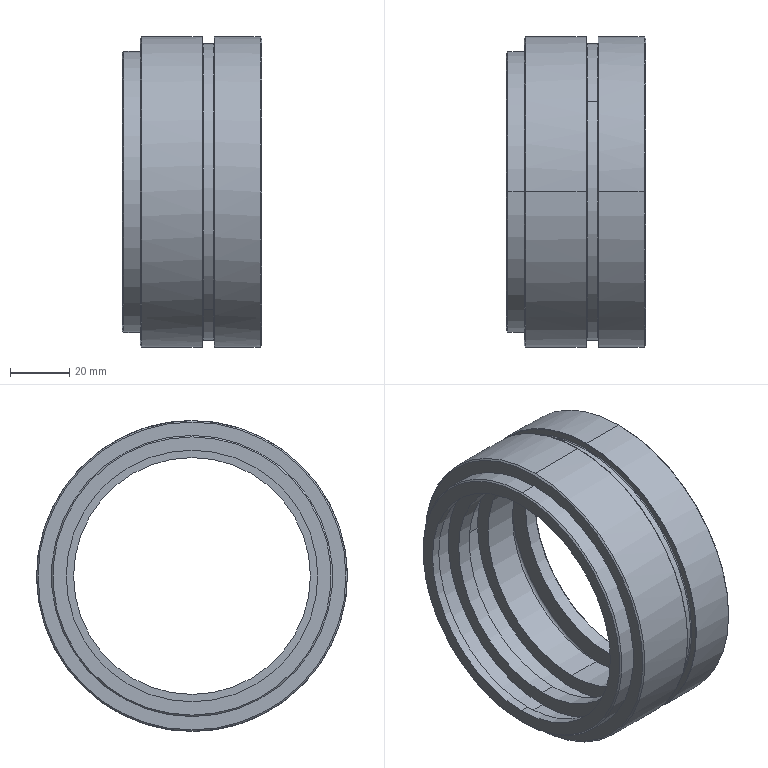Part | SolidWorks | features Cavity 1, Chamfer 1, Extrusion 1, ICE 1 | 1 solid | 53 faces | box 47 x 105 x 105 mm | volume 121428 mm3 | cylinder 22 | torus 12 | plane 11 | cone 8 | commonest cylinder face diameters 80 x6 90 x4 105 x4 85 x2 95 x2 95.5 x2
STEP:
#1=CARTESIAN_POINT('',(35.7,0.,-40.));
#2=VERTEX_POINT('',#1);
#3=CARTESIAN_POINT('',(35.7,0.,40.));
#4=VERTEX_POINT('',#3);
#5=CARTESIAN_POINT('',(35.7,0.000000867,0.000001335));
#6=DIRECTION('',(-1.,0.,0.));
#7=DIRECTION('',(0.,-0.1106,0.9939));
#8=AXIS2_PLACEMENT_3D('',#5,#6,#7);
#9=CIRCLE('',#8,40.);
#10=EDGE_CURVE('',#2,#4,#9,.T.);
#11=ORIENTED_EDGE('',*,*,#10,.F.);
#12=CARTESIAN_POINT('',(24.,0.,-40.));
#13=VERTEX_POINT('',#12);
#14=CARTESIAN_POINT('',(47.,0.,-40.));
#15=DIRECTION('',(-1.,0.,0.));
#16=VECTOR('',#15,1000.);
#17=LINE('',#14,#16);
#18=EDGE_CURVE('',#2,#13,#17,.T.);
#19=ORIENTED_EDGE('',*,*,#18,.T.);
#20=CARTESIAN_POINT('',(24.,0.,40.));
#21=VERTEX_POINT('',#20);
#22=CARTESIAN_POINT('',(24.,0.000000867,0.000001335));
#23=DIRECTION('',(-1.,0.,0.));
#24=DIRECTION('',(0.,-0.9995,0.03037));
#25=AXIS2_PLACEMENT_3D('',#22,#23,#24);
#26=CIRCLE('',#25,40.);
#27=EDGE_CURVE('',#13,#21,#26,.T.);
#28=ORIENTED_EDGE('',*,*,#27,.T.);
#29=CARTESIAN_POINT('',(47.,0.,40.));
#30=DIRECTION('',(-1.,0.,0.));
#31=VECTOR('',#30,1000.);
#32=LINE('',#29,#31);
#33=EDGE_CURVE('',#4,#21,#32,.T.);
#34=ORIENTED_EDGE('',*,*,#33,.F.);
#35=EDGE_LOOP('',(#11,#19,#28,#34));
#36=FACE_OUTER_BOUND('',#35,.T.);
#37=CARTESIAN_POINT('',(47.,0.,0.));
#38=DIRECTION('',(-1.,0.,0.));
#39=DIRECTION('',(0.,0.,1.));
#40=AXIS2_PLACEMENT_3D('',#37,#38,#39);
#41=CYLINDRICAL_SURFACE('',#40,40.);
#42=ADVANCED_FACE('',(#36),#41,.F.);
#43=CARTESIAN_POINT('',(24.,44.979,-1.366));
#44=VERTEX_POINT('',#43);
#45=CARTESIAN_POINT('',(24.,-44.979,1.366));
#46=VERTEX_POINT('',#45);
#47=CARTESIAN_POINT('',(24.,0.000000867,0.000001335));
#48=DIRECTION('',(-1.,0.,0.));
#49=DIRECTION('',(0.,-0.9995,0.03037));
#50=AXIS2_PLACEMENT_3D('',#47,#48,#49);
#51=CIRCLE('',#50,45.);
#52=EDGE_CURVE('',#44,#46,#51,.T.);
#53=ORIENTED_EDGE('',*,*,#52,.F.);
#54=CARTESIAN_POINT('',(15.,44.979,-1.366));
#55=VERTEX_POINT('',#54);
#56=CARTESIAN_POINT('',(15.,44.979,-1.366));
#57=DIRECTION('',(-1.,0.,0.));
#58=VECTOR('',#57,1000.);
#59=LINE('',#56,#58);
#60=EDGE_CURVE('',#44,#55,#59,.T.);
#61=ORIENTED_EDGE('',*,*,#60,.T.);
#62=CARTESIAN_POINT('',(15.,-44.979,1.366));
#63=VERTEX_POINT('',#62);
#64=CARTESIAN_POINT('',(15.,0.000000867,0.000001335));
#65=DIRECTION('',(-1.,0.,0.));
#66=DIRECTION('',(0.,-0.9995,0.03037));
#67=AXIS2_PLACEMENT_3D('',#64,#65,#66);
#68=CIRCLE('',#67,45.);
#69=EDGE_CURVE('',#55,#63,#68,.T.);
#70=ORIENTED_EDGE('',*,*,#69,.T.);
#71=CARTESIAN_POINT('',(15.,-44.979,1.366));
#72=DIRECTION('',(-1.,0.,0.));
#73=VECTOR('',#72,1000.);
#74=LINE('',#71,#73);
#75=EDGE_CURVE('',#46,#63,#74,.T.);
#76=ORIENTED_EDGE('',*,*,#75,.F.);
#77=EDGE_LOOP('',(#53,#61,#70,#76));
#78=FACE_OUTER_BOUND('',#77,.T.);
#79=CARTESIAN_POINT('',(15.,0.000000867,0.000001335));
#80=DIRECTION('',(-1.,0.,0.));
#81=DIRECTION('',(0.,-0.9995,0.03037));
#82=AXIS2_PLACEMENT_3D('',#79,#80,#81);
#83=CYLINDRICAL_SURFACE('',#82,45.);
#84=ADVANCED_FACE('',(#78),#83,.F.);
#85=CARTESIAN_POINT('',(36.7,5.281,-47.457));
#86=VERTEX_POINT('',#85);
#87=CARTESIAN_POINT('',(36.7,-5.281,47.457));
#88=VERTEX_POINT('',#87);
#89=CARTESIAN_POINT('',(36.7,0.000000867,0.000001335));
#90=DIRECTION('',(-1.,0.,0.));
#91=DIRECTION('',(0.,-0.1106,0.9939));
#92=AXIS2_PLACEMENT_3D('',#89,#90,#91);
#93=CIRCLE('',#92,47.75);
#94=EDGE_CURVE('',#86,#88,#93,.T.);
#95=ORIENTED_EDGE('',*,*,#94,.F.);
#96=CARTESIAN_POINT('',(35.7,5.171,-46.463));
#97=VERTEX_POINT('',#96);
#98=CARTESIAN_POINT('',(36.7,5.171,-46.463));
#99=DIRECTION('',(0.,0.9939,0.1106));
#100=DIRECTION('',(0.,-0.1106,0.9939));
#101=AXIS2_PLACEMENT_3D('',#98,#99,#100);
#102=CIRCLE('',#101,1.);
#103=EDGE_CURVE('',#86,#97,#102,.T.);
#104=ORIENTED_EDGE('',*,*,#103,.T.);
#105=CARTESIAN_POINT('',(35.7,-5.171,46.463));
#106=VERTEX_POINT('',#105);
#107=CARTESIAN_POINT('',(35.7,0.000000867,0.000001335));
#108=DIRECTION('',(-1.,0.,0.));
#109=DIRECTION('',(0.,-0.1106,0.9939));
#110=AXIS2_PLACEMENT_3D('',#107,#108,#109);
#111=CIRCLE('',#110,46.75);
#112=EDGE_CURVE('',#97,#106,#111,.T.);
#113=ORIENTED_EDGE('',*,*,#112,.T.);
#114=CARTESIAN_POINT('',(36.7,-5.171,46.463));
#115=DIRECTION('',(0.,-0.9939,-0.1106));
#116=DIRECTION('',(0.,0.1106,-0.9939));
#117=AXIS2_PLACEMENT_3D('',#114,#115,#116);
#118=CIRCLE('',#117,1.);
#119=EDGE_CURVE('',#88,#106,#118,.T.);
#120=ORIENTED_EDGE('',*,*,#119,.F.);
#121=EDGE_LOOP('',(#95,#104,#113,#120));
#122=FACE_OUTER_BOUND('',#121,.T.);
#123=CARTESIAN_POINT('',(36.7,0.000000867,0.000001335));
#124=DIRECTION('',(-1.,0.,0.));
#125=DIRECTION('',(0.,-0.1106,0.9939));
#126=AXIS2_PLACEMENT_3D('',#123,#124,#125);
#127=TOROIDAL_SURFACE('',#126,46.75,1.);
#128=ADVANCED_FACE('',(#122),#127,.F.);
#129=CARTESIAN_POINT('',(41.,5.281,-47.457));
#130=VERTEX_POINT('',#129);
#131=CARTESIAN_POINT('',(41.,-5.281,47.457));
#132=VERTEX_POINT('',#131);
#133=CARTESIAN_POINT('',(41.,0.000000867,0.000001335));
#134=DIRECTION('',(-1.,0.,0.));
#135=DIRECTION('',(0.,-0.1106,0.9939));
#136=AXIS2_PLACEMENT_3D('',#133,#134,#135);
#137=CIRCLE('',#136,47.75);
#138=EDGE_CURVE('',#130,#132,#137,.T.);
#139=ORIENTED_EDGE('',*,*,#138,.F.);
#140=CARTESIAN_POINT('',(35.7,5.281,-47.457));
#141=DIRECTION('',(-1.,0.,0.));
#142=VECTOR('',#141,1000.);
#143=LINE('',#140,#142);
#144=EDGE_CURVE('',#130,#86,#143,.T.);
#145=ORIENTED_EDGE('',*,*,#144,.T.);
#146=ORIENTED_EDGE('',*,*,#94,.T.);
#147=CARTESIAN_POINT('',(35.7,-5.281,47.457));
#148=DIRECTION('',(-1.,0.,0.));
#149=VECTOR('',#148,1000.);
#150=LINE('',#147,#149);
#151=EDGE_CURVE('',#132,#88,#150,.T.);
#152=ORIENTED_EDGE('',*,*,#151,.F.);
#153=EDGE_LOOP('',(#139,#145,#146,#152));
#154=FACE_OUTER_BOUND('',#153,.T.);
#155=CARTESIAN_POINT('',(35.7,0.000000867,0.000001335));
#156=DIRECTION('',(-1.,0.,0.));
#157=DIRECTION('',(0.,-0.1106,0.9939));
#158=AXIS2_PLACEMENT_3D('',#155,#156,#157);
#159=CYLINDRICAL_SURFACE('',#158,47.75);
#160=ADVANCED_FACE('',(#154),#159,.F.);
#161=CARTESIAN_POINT('',(42.,5.171,-46.463));
#162=VERTEX_POINT('',#161);
#163=CARTESIAN_POINT('',(42.,-5.171,46.463));
#164=VERTEX_POINT('',#163);
#165=CARTESIAN_POINT('',(42.,0.000000867,0.000001335));
#166=DIRECTION('',(-1.,0.,0.));
#167=DIRECTION('',(0.,-0.1106,0.9939));
#168=AXIS2_PLACEMENT_3D('',#165,#166,#167);
#169=CIRCLE('',#168,46.75);
#170=EDGE_CURVE('',#162,#164,#169,.T.);
#171=ORIENTED_EDGE('',*,*,#170,.F.);
#172=CARTESIAN_POINT('',(41.,5.171,-46.463));
#173=DIRECTION('',(0.,0.9939,0.1106));
#174=DIRECTION('',(0.,-0.1106,0.9939));
#175=AXIS2_PLACEMENT_3D('',#172,#173,#174);
#176=CIRCLE('',#175,1.);
#177=EDGE_CURVE('',#162,#130,#176,.T.);
#178=ORIENTED_EDGE('',*,*,#177,.T.);
#179=ORIENTED_EDGE('',*,*,#138,.T.);
#180=CARTESIAN_POINT('',(41.,-5.171,46.463));
#181=DIRECTION('',(0.,-0.9939,-0.1106));
#182=DIRECTION('',(0.,0.1106,-0.9939));
#183=AXIS2_PLACEMENT_3D('',#180,#181,#182);
#184=CIRCLE('',#183,1.);
#185=EDGE_CURVE('',#164,#132,#184,.T.);
#186=ORIENTED_EDGE('',*,*,#185,.F.);
#187=EDGE_LOOP('',(#171,#178,#179,#186));
#188=FACE_OUTER_BOUND('',#187,.T.);
#189=CARTESIAN_POINT('',(41.,0.000000867,0.000001335));
#190=DIRECTION('',(-1.,0.,0.));
#191=DIRECTION('',(0.,-0.1106,0.9939));
#192=AXIS2_PLACEMENT_3D('',#189,#190,#191);
#193=TOROIDAL_SURFACE('',#192,46.75,1.);
#194=ADVANCED_FACE('',(#188),#193,.F.);
#195=CARTESIAN_POINT('',(46.5,0.,40.));
#196=VERTEX_POINT('',#195);
#197=CARTESIAN_POINT('',(46.5,0.,-40.));
#198=VERTEX_POINT('',#197);
#199=CARTESIAN_POINT('',(46.5,0.,0.));
#200=DIRECTION('',(1.,0.,0.));
#201=DIRECTION('',(0.,0.,-1.));
#202=AXIS2_PLACEMENT_3D('',#199,#200,#201);
#203=CIRCLE('',#202,40.);
#204=EDGE_CURVE('',#196,#198,#203,.T.);
#205=ORIENTED_EDGE('',*,*,#204,.T.);
#206=CARTESIAN_POINT('',(42.,0.,-40.));
#207=VERTEX_POINT('',#206);
#208=CARTESIAN_POINT('',(47.,0.,-40.));
#209=DIRECTION('',(-1.,0.,0.));
#210=VECTOR('',#209,1000.);
#211=LINE('',#208,#210);
#212=EDGE_CURVE('',#198,#207,#211,.T.);
#213=ORIENTED_EDGE('',*,*,#212,.T.);
#214=CARTESIAN_POINT('',(42.,0.,40.));
#215=VERTEX_POINT('',#214);
#216=CARTESIAN_POINT('',(42.,0.000000867,0.000001335));
#217=DIRECTION('',(-1.,0.,0.));
#218=DIRECTION('',(0.,-0.1106,0.9939));
#219=AXIS2_PLACEMENT_3D('',#216,#217,#218);
#220=CIRCLE('',#219,40.);
#221=EDGE_CURVE('',#207,#215,#220,.T.);
#222=ORIENTED_EDGE('',*,*,#221,.T.);
#223=CARTESIAN_POINT('',(47.,0.,40.));
#224=DIRECTION('',(-1.,0.,0.));
#225=VECTOR('',#224,1000.);
#226=LINE('',#223,#225);
#227=EDGE_CURVE('',#196,#215,#226,.T.);
#228=ORIENTED_EDGE('',*,*,#227,.F.);
#229=EDGE_LOOP('',(#205,#213,#222,#228));
#230=FACE_OUTER_BOUND('',#229,.T.);
#231=CARTESIAN_POINT('',(47.,0.,0.));
#232=DIRECTION('',(-1.,0.,0.));
#233=DIRECTION('',(0.,0.,1.));
#234=AXIS2_PLACEMENT_3D('',#231,#232,#233);
#235=CYLINDRICAL_SURFACE('',#234,40.);
#236=ADVANCED_FACE('',(#230),#235,.F.);
#237=ORIENTED_EDGE('',*,*,#204,.F.);
#238=CARTESIAN_POINT('',(47.,0.,40.5));
#239=VERTEX_POINT('',#238);
#240=CARTESIAN_POINT('',(46.5,0.,40.));
#241=DIRECTION('',(0.7071,0.,0.7071));
#242=VECTOR('',#241,1000.);
#243=LINE('',#240,#242);
#244=EDGE_CURVE('',#196,#239,#243,.T.);
#245=ORIENTED_EDGE('',*,*,#244,.T.);
#246=CARTESIAN_POINT('',(47.,0.,-40.5));
#247=VERTEX_POINT('',#246);
#248=CARTESIAN_POINT('',(47.,0.,0.));
#249=DIRECTION('',(-1.,0.,0.));
#250=DIRECTION('',(0.,0.,-1.));
#251=AXIS2_PLACEMENT_3D('',#248,#249,#250);
#252=CIRCLE('',#251,40.5);
#253=EDGE_CURVE('',#247,#239,#252,.T.);
#254=ORIENTED_EDGE('',*,*,#253,.F.);
#255=CARTESIAN_POINT('',(46.5,0.,-40.));
#256=DIRECTION('',(0.7071,0.,-0.7071));
#257=VECTOR('',#256,1000.);
#258=LINE('',#255,#257);
#259=EDGE_CURVE('',#198,#247,#258,.T.);
#260=ORIENTED_EDGE('',*,*,#259,.F.);
#261=EDGE_LOOP('',(#237,#245,#254,#260));
#262=FACE_OUTER_BOUND('',#261,.T.);
#263=CARTESIAN_POINT('',(46.5,0.,0.));
#264=DIRECTION('',(1.,0.,0.));
#265=DIRECTION('',(0.,0.,-1.));
#266=AXIS2_PLACEMENT_3D('',#263,#264,#265);
#267=CONICAL_SURFACE('',#266,40.,0.7854);
#268=ADVANCED_FACE('',(#262),#267,.F.);
#269=CARTESIAN_POINT('',(46.5,0.,52.5));
#270=VERTEX_POINT('',#269);
#271=CARTESIAN_POINT('',(46.5,0.,-52.5));
#272=VERTEX_POINT('',#271);
#273=CARTESIAN_POINT('',(46.5,0.,0.));
#274=DIRECTION('',(-1.,0.,0.));
#275=DIRECTION('',(0.,0.,-1.));
#276=AXIS2_PLACEMENT_3D('',#273,#274,#275);
#277=CIRCLE('',#276,52.5);
#278=EDGE_CURVE('',#270,#272,#277,.T.);
#279=ORIENTED_EDGE('',*,*,#278,.T.);
#280=CARTESIAN_POINT('',(31.1,0.,-52.5));
#281=VERTEX_POINT('',#280);
#282=CARTESIAN_POINT('',(47.,0.,-52.5));
#283=DIRECTION('',(-1.,0.,0.));
#284=VECTOR('',#283,1000.);
#285=LINE('',#282,#284);
#286=EDGE_CURVE('',#272,#281,#285,.T.);
#287=ORIENTED_EDGE('',*,*,#286,.T.);
#288=CARTESIAN_POINT('',(31.1,31.96,41.651));
#289=VERTEX_POINT('',#288);
#290=CARTESIAN_POINT('',(31.1,0.,0.));
#291=DIRECTION('',(1.,0.,0.));
#292=DIRECTION('',(0.,-0.6088,-0.7934));
#293=AXIS2_PLACEMENT_3D('',#290,#291,#292);
#294=CIRCLE('',#293,52.5);
#295=EDGE_CURVE('',#281,#289,#294,.T.);
#296=ORIENTED_EDGE('',*,*,#295,.T.);
#297=CARTESIAN_POINT('',(31.1,0.,52.5));
#298=VERTEX_POINT('',#297);
#299=CARTESIAN_POINT('',(31.1,0.,0.));
#300=DIRECTION('',(1.,0.,0.));
#301=DIRECTION('',(0.,-0.6088,-0.7934));
#302=AXIS2_PLACEMENT_3D('',#299,#300,#301);
#303=CIRCLE('',#302,52.5);
#304=EDGE_CURVE('',#289,#298,#303,.T.);
#305=ORIENTED_EDGE('',*,*,#304,.T.);
#306=CARTESIAN_POINT('',(47.,0.,52.5));
#307=DIRECTION('',(-1.,0.,0.));
#308=VECTOR('',#307,1000.);
#309=LINE('',#306,#308);
#310=EDGE_CURVE('',#270,#298,#309,.T.);
#311=ORIENTED_EDGE('',*,*,#310,.F.);
#312=EDGE_LOOP('',(#279,#287,#296,#305,#311));
#313=FACE_OUTER_BOUND('',#312,.T.);
#314=CARTESIAN_POINT('',(47.,0.,0.));
#315=DIRECTION('',(-1.,0.,0.));
#316=DIRECTION('',(0.,0.,1.));
#317=AXIS2_PLACEMENT_3D('',#314,#315,#316);
#318=CYLINDRICAL_SURFACE('',#317,52.5);
#319=ADVANCED_FACE('',(#313),#318,.T.);
#320=CARTESIAN_POINT('',(47.,0.,-52.));
#321=VERTEX_POINT('',#320);
#322=CARTESIAN_POINT('',(47.,0.,52.));
#323=VERTEX_POINT('',#322);
#324=CARTESIAN_POINT('',(47.,0.,0.));
#325=DIRECTION('',(1.,0.,0.));
#326=DIRECTION('',(0.,0.,-1.));
#327=AXIS2_PLACEMENT_3D('',#324,#325,#326);
#328=CIRCLE('',#327,52.);
#329=EDGE_CURVE('',#321,#323,#328,.T.);
#330=ORIENTED_EDGE('',*,*,#329,.F.);
#331=CARTESIAN_POINT('',(47.,0.,-52.));
#332=DIRECTION('',(-0.7071,0.,-0.7071));
#333=VECTOR('',#332,1000.);
#334=LINE('',#331,#333);
#335=EDGE_CURVE('',#321,#272,#334,.T.);
#336=ORIENTED_EDGE('',*,*,#335,.T.);
#337=ORIENTED_EDGE('',*,*,#278,.F.);
#338=CARTESIAN_POINT('',(47.,0.,52.));
#339=DIRECTION('',(-0.7071,0.,0.7071));
#340=VECTOR('',#339,1000.);
#341=LINE('',#338,#340);
#342=EDGE_CURVE('',#323,#270,#341,.T.);
#343=ORIENTED_EDGE('',*,*,#342,.F.);
#344=EDGE_LOOP('',(#330,#336,#337,#343));
#345=FACE_OUTER_BOUND('',#344,.T.);
#346=CARTESIAN_POINT('',(47.,0.,0.));
#347=DIRECTION('',(-1.,0.,0.));
#348=DIRECTION('',(0.,0.,1.));
#349=AXIS2_PLACEMENT_3D('',#346,#347,#348);
#350=CONICAL_SURFACE('',#349,52.,0.7854);
#351=ADVANCED_FACE('',(#345),#350,.T.);
#352=CARTESIAN_POINT('',(15.,0.,-40.));
#353=VERTEX_POINT('',#352);
#354=CARTESIAN_POINT('',(15.,0.,40.));
#355=VERTEX_POINT('',#354);
#356=CARTESIAN_POINT('',(15.,0.000000867,0.000001335));
#357=DIRECTION('',(-1.,0.,0.));
#358=DIRECTION('',(0.,-0.9995,0.03037));
#359=AXIS2_PLACEMENT_3D('',#356,#357,#358);
#360=CIRCLE('',#359,40.);
#361=EDGE_CURVE('',#353,#355,#360,.T.);
#362=ORIENTED_EDGE('',*,*,#361,.F.);
#363=CARTESIAN_POINT('',(10.,0.,-40.));
#364=VERTEX_POINT('',#363);
#365=CARTESIAN_POINT('',(47.,0.,-40.));
#366=DIRECTION('',(-1.,0.,0.));
#367=VECTOR('',#366,1000.);
#368=LINE('',#365,#367);
#369=EDGE_CURVE('',#353,#364,#368,.T.);
#370=ORIENTED_EDGE('',*,*,#369,.T.);
#371=CARTESIAN_POINT('',(10.,0.,40.));
#372=VERTEX_POINT('',#371);
#373=CARTESIAN_POINT('',(10.,0.,0.));
#374=DIRECTION('',(-1.,0.,0.));
#375=DIRECTION('',(0.,0.,1.));
#376=AXIS2_PLACEMENT_3D('',#373,#374,#375);
#377=CIRCLE('',#376,40.);
#378=EDGE_CURVE('',#364,#372,#377,.T.);
#379=ORIENTED_EDGE('',*,*,#378,.T.);
#380=CARTESIAN_POINT('',(47.,0.,40.));
#381=DIRECTION('',(-1.,0.,0.));
#382=VECTOR('',#381,1000.);
#383=LINE('',#380,#382);
#384=EDGE_CURVE('',#355,#372,#383,.T.);
#385=ORIENTED_EDGE('',*,*,#384,.F.);
#386=EDGE_LOOP('',(#362,#370,#379,#385));
#387=FACE_OUTER_BOUND('',#386,.T.);
#388=CARTESIAN_POINT('',(47.,0.,0.));
#389=DIRECTION('',(-1.,0.,0.));
#390=DIRECTION('',(0.,0.,1.));
#391=AXIS2_PLACEMENT_3D('',#388,#389,#390);
#392=CYLINDRICAL_SURFACE('',#391,40.);
#393=ADVANCED_FACE('',(#387),#392,.F.);
#394=CARTESIAN_POINT('',(31.,-31.899,-41.572));
#395=VERTEX_POINT('',#394);
#396=CARTESIAN_POINT('',(31.,31.899,41.572));
#397=VERTEX_POINT('',#396);
#398=CARTESIAN_POINT('',(31.,0.,0.));
#399=DIRECTION('',(1.,0.,0.));
#400=DIRECTION('',(0.,-0.6088,-0.7934));
#401=AXIS2_PLACEMENT_3D('',#398,#399,#400);
#402=CIRCLE('',#401,52.4);
#403=EDGE_CURVE('',#395,#397,#402,.T.);
#404=ORIENTED_EDGE('',*,*,#403,.T.);
#405=CARTESIAN_POINT('',(31.1,31.899,41.572));
#406=DIRECTION('',(0.,0.7934,-0.6088));
#407=DIRECTION('',(0.,0.6088,0.7934));
#408=AXIS2_PLACEMENT_3D('',#405,#406,#407);
#409=CIRCLE('',#408,0.1);
#410=EDGE_CURVE('',#397,#289,#409,.T.);
#411=ORIENTED_EDGE('',*,*,#410,.T.);
#412=ORIENTED_EDGE('',*,*,#295,.F.);
#413=CARTESIAN_POINT('',(31.1,-31.96,-41.651));
#414=VERTEX_POINT('',#413);
#415=CARTESIAN_POINT('',(31.1,0.,0.));
#416=DIRECTION('',(1.,0.,0.));
#417=DIRECTION('',(0.,-0.6088,-0.7934));
#418=AXIS2_PLACEMENT_3D('',#415,#416,#417);
#419=CIRCLE('',#418,52.5);
#420=EDGE_CURVE('',#414,#281,#419,.T.);
#421=ORIENTED_EDGE('',*,*,#420,.F.);
#422=CARTESIAN_POINT('',(31.1,-31.899,-41.572));
#423=DIRECTION('',(0.,-0.7934,0.6088));
#424=DIRECTION('',(0.,-0.6088,-0.7934));
#425=AXIS2_PLACEMENT_3D('',#422,#423,#424);
#426=CIRCLE('',#425,0.1);
#427=EDGE_CURVE('',#395,#414,#426,.T.);
#428=ORIENTED_EDGE('',*,*,#427,.F.);
#429=EDGE_LOOP('',(#404,#411,#412,#421,#428));
#430=FACE_OUTER_BOUND('',#429,.T.);
#431=CARTESIAN_POINT('',(31.1,0.,0.));
#432=DIRECTION('',(1.,0.,0.));
#433=DIRECTION('',(0.,-0.6088,-0.7934));
#434=AXIS2_PLACEMENT_3D('',#431,#432,#433);
#435=TOROIDAL_SURFACE('',#434,52.4,0.1);
#436=ADVANCED_FACE('',(#430),#435,.T.);
#437=CARTESIAN_POINT('',(26.9,0.,-52.5));
#438=VERTEX_POINT('',#437);
#439=CARTESIAN_POINT('',(26.9,31.96,41.651));
#440=VERTEX_POINT('',#439);
#441=CARTESIAN_POINT('',(26.9,0.,0.));
#442=DIRECTION('',(1.,0.,0.));
#443=DIRECTION('',(0.,-0.6088,-0.7934));
#444=AXIS2_PLACEMENT_3D('',#441,#442,#443);
#445=CIRCLE('',#444,52.5);
#446=EDGE_CURVE('',#438,#440,#445,.T.);
#447=ORIENTED_EDGE('',*,*,#446,.T.);
#448=CARTESIAN_POINT('',(27.,31.899,41.572));
#449=VERTEX_POINT('',#448);
#450=CARTESIAN_POINT('',(26.9,31.899,41.572));
#451=DIRECTION('',(0.,0.7934,-0.6088));
#452=DIRECTION('',(0.,0.6088,0.7934));
#453=AXIS2_PLACEMENT_3D('',#450,#451,#452);
#454=CIRCLE('',#453,0.1);
#455=EDGE_CURVE('',#440,#449,#454,.T.);
#456=ORIENTED_EDGE('',*,*,#455,.T.);
#457=CARTESIAN_POINT('',(27.,-31.899,-41.572));
#458=VERTEX_POINT('',#457);
#459=CARTESIAN_POINT('',(27.,0.,0.));
#460=DIRECTION('',(1.,0.,0.));
#461=DIRECTION('',(0.,-0.6088,-0.7934));
#462=AXIS2_PLACEMENT_3D('',#459,#460,#461);
#463=CIRCLE('',#462,52.4);
#464=EDGE_CURVE('',#458,#449,#463,.T.);
#465=ORIENTED_EDGE('',*,*,#464,.F.);
#466=CARTESIAN_POINT('',(26.9,-31.96,-41.651));
#467=VERTEX_POINT('',#466);
#468=CARTESIAN_POINT('',(26.9,-31.899,-41.572));
#469=DIRECTION('',(0.,-0.7934,0.6088));
#470=DIRECTION('',(0.,-0.6088,-0.7934));
#471=AXIS2_PLACEMENT_3D('',#468,#469,#470);
#472=CIRCLE('',#471,0.1);
#473=EDGE_CURVE('',#467,#458,#472,.T.);
#474=ORIENTED_EDGE('',*,*,#473,.F.);
#475=CARTESIAN_POINT('',(26.9,0.,0.));
#476=DIRECTION('',(1.,0.,0.));
#477=DIRECTION('',(0.,-0.6088,-0.7934));
#478=AXIS2_PLACEMENT_3D('',#475,#476,#477);
#479=CIRCLE('',#478,52.5);
#480=EDGE_CURVE('',#467,#438,#479,.T.);
#481=ORIENTED_EDGE('',*,*,#480,.T.);
#482=EDGE_LOOP('',(#447,#456,#465,#474,#481));
#483=FACE_OUTER_BOUND('',#482,.T.);
#484=CARTESIAN_POINT('',(26.9,0.,0.));
#485=DIRECTION('',(1.,0.,0.));
#486=DIRECTION('',(0.,-0.6088,-0.7934));
#487=AXIS2_PLACEMENT_3D('',#484,#485,#486);
#488=TOROIDAL_SURFACE('',#487,52.4,0.1);
#489=ADVANCED_FACE('',(#483),#488,.T.);
#490=CARTESIAN_POINT('',(27.3,30.499,39.747));
#491=VERTEX_POINT('',#490);
#492=CARTESIAN_POINT('',(27.3,-30.499,-39.747));
#493=VERTEX_POINT('',#492);
#494=CARTESIAN_POINT('',(27.3,0.,0.));
#495=DIRECTION('',(1.,0.,0.));
#496=DIRECTION('',(0.,-0.6088,-0.7934));
#497=AXIS2_PLACEMENT_3D('',#494,#495,#496);
#498=CIRCLE('',#497,50.1);
#499=EDGE_CURVE('',#491,#493,#498,.T.);
#500=ORIENTED_EDGE('',*,*,#499,.F.);
#501=CARTESIAN_POINT('',(27.,30.681,39.985));
#502=VERTEX_POINT('',#501);
#503=CARTESIAN_POINT('',(27.3,30.681,39.985));
#504=DIRECTION('',(0.,0.7934,-0.6088));
#505=DIRECTION('',(0.,0.6088,0.7934));
#506=AXIS2_PLACEMENT_3D('',#503,#504,#505);
#507=CIRCLE('',#506,0.3);
#508=EDGE_CURVE('',#491,#502,#507,.T.);
#509=ORIENTED_EDGE('',*,*,#508,.T.);
#510=CARTESIAN_POINT('',(27.,-30.681,-39.985));
#511=VERTEX_POINT('',#510);
#512=CARTESIAN_POINT('',(27.,0.,0.));
#513=DIRECTION('',(1.,0.,0.));
#514=DIRECTION('',(0.,-0.6088,-0.7934));
#515=AXIS2_PLACEMENT_3D('',#512,#513,#514);
#516=CIRCLE('',#515,50.4);
#517=EDGE_CURVE('',#502,#511,#516,.T.);
#518=ORIENTED_EDGE('',*,*,#517,.T.);
#519=CARTESIAN_POINT('',(27.3,-30.681,-39.985));
#520=DIRECTION('',(0.,-0.7934,0.6088));
#521=DIRECTION('',(0.,-0.6088,-0.7934));
#522=AXIS2_PLACEMENT_3D('',#519,#520,#521);
#523=CIRCLE('',#522,0.3);
#524=EDGE_CURVE('',#493,#511,#523,.T.);
#525=ORIENTED_EDGE('',*,*,#524,.F.);
#526=EDGE_LOOP('',(#500,#509,#518,#525));
#527=FACE_OUTER_BOUND('',#526,.T.);
#528=CARTESIAN_POINT('',(27.3,0.,0.));
#529=DIRECTION('',(1.,0.,0.));
#530=DIRECTION('',(0.,-0.6088,-0.7934));
#531=AXIS2_PLACEMENT_3D('',#528,#529,#530);
#532=TOROIDAL_SURFACE('',#531,50.4,0.3);
#533=ADVANCED_FACE('',(#527),#532,.F.);
#534=CARTESIAN_POINT('',(27.3,0.,0.));
#535=DIRECTION('',(1.,0.,0.));
#536=DIRECTION('',(0.,-0.6088,-0.7934));
#537=AXIS2_PLACEMENT_3D('',#534,#535,#536);
#538=CIRCLE('',#537,50.1);
#539=EDGE_CURVE('',#493,#491,#538,.T.);
#540=ORIENTED_EDGE('',*,*,#539,.T.);
#541=CARTESIAN_POINT('',(30.7,30.499,39.747));
#542=VERTEX_POINT('',#541);
#543=CARTESIAN_POINT('',(196.04,30.499,39.747));
#544=DIRECTION('',(1.,0.,0.));
#545=VECTOR('',#544,1000.);
#546=LINE('',#543,#545);
#547=EDGE_CURVE('',#491,#542,#546,.T.);
#548=ORIENTED_EDGE('',*,*,#547,.T.);
#549=CARTESIAN_POINT('',(30.7,-30.499,-39.747));
#550=VERTEX_POINT('',#549);
#551=CARTESIAN_POINT('',(30.7,0.,0.));
#552=DIRECTION('',(1.,0.,0.));
#553=DIRECTION('',(0.,-0.6088,-0.7934));
#554=AXIS2_PLACEMENT_3D('',#551,#552,#553);
#555=CIRCLE('',#554,50.1);
#556=EDGE_CURVE('',#550,#542,#555,.T.);
#557=ORIENTED_EDGE('',*,*,#556,.F.);
#558=CARTESIAN_POINT('',(196.04,-30.499,-39.747));
#559=DIRECTION('',(1.,0.,0.));
#560=VECTOR('',#559,1000.);
#561=LINE('',#558,#560);
#562=EDGE_CURVE('',#493,#550,#561,.T.);
#563=ORIENTED_EDGE('',*,*,#562,.F.);
#564=EDGE_LOOP('',(#540,#548,#557,#563));
#565=FACE_OUTER_BOUND('',#564,.T.);
#566=CARTESIAN_POINT('',(196.04,0.,0.));
#567=DIRECTION('',(1.,0.,0.));
#568=DIRECTION('',(0.,-0.6088,-0.7934));
#569=AXIS2_PLACEMENT_3D('',#566,#567,#568);
#570=CYLINDRICAL_SURFACE('',#569,50.1);
#571=ADVANCED_FACE('',(#565),#570,.T.);
#572=CARTESIAN_POINT('',(31.,30.681,39.985));
#573=VERTEX_POINT('',#572);
#574=CARTESIAN_POINT('',(31.,-30.681,-39.985));
#575=VERTEX_POINT('',#574);
#576=CARTESIAN_POINT('',(31.,0.,0.));
#577=DIRECTION('',(1.,0.,0.));
#578=DIRECTION('',(0.,-0.6088,-0.7934));
#579=AXIS2_PLACEMENT_3D('',#576,#577,#578);
#580=CIRCLE('',#579,50.4);
#581=EDGE_CURVE('',#573,#575,#580,.T.);
#582=ORIENTED_EDGE('',*,*,#581,.F.);
#583=CARTESIAN_POINT('',(30.7,30.681,39.985));
#584=DIRECTION('',(0.,0.7934,-0.6088));
#585=DIRECTION('',(0.,0.6088,0.7934));
#586=AXIS2_PLACEMENT_3D('',#583,#584,#585);
#587=CIRCLE('',#586,0.3);
#588=EDGE_CURVE('',#573,#542,#587,.T.);
#589=ORIENTED_EDGE('',*,*,#588,.T.);
#590=CARTESIAN_POINT('',(30.7,0.,0.));
#591=DIRECTION('',(1.,0.,0.));
#592=DIRECTION('',(0.,-0.6088,-0.7934));
#593=AXIS2_PLACEMENT_3D('',#590,#591,#592);
#594=CIRCLE('',#593,50.1);
#595=EDGE_CURVE('',#542,#550,#594,.T.);
#596=ORIENTED_EDGE('',*,*,#595,.T.);
#597=CARTESIAN_POINT('',(30.7,-30.681,-39.985));
#598=DIRECTION('',(0.,-0.7934,0.6088));
#599=DIRECTION('',(0.,-0.6088,-0.7934));
#600=AXIS2_PLACEMENT_3D('',#597,#598,#599);
#601=CIRCLE('',#600,0.3);
#602=EDGE_CURVE('',#575,#550,#601,.T.);
#603=ORIENTED_EDGE('',*,*,#602,.F.);
#604=EDGE_LOOP('',(#582,#589,#596,#603));
#605=FACE_OUTER_BOUND('',#604,.T.);
#606=CARTESIAN_POINT('',(30.7,0.,0.));
#607=DIRECTION('',(1.,0.,0.));
#608=DIRECTION('',(0.,-0.6088,-0.7934));
#609=AXIS2_PLACEMENT_3D('',#606,#607,#608);
#610=TOROIDAL_SURFACE('',#609,50.4,0.3);
#611=ADVANCED_FACE('',(#605),#610,.F.);
#612=CARTESIAN_POINT('',(10.,0.,-45.));
#613=VERTEX_POINT('',#612);
#614=CARTESIAN_POINT('',(10.,0.,45.));
#615=VERTEX_POINT('',#614);
#616=CARTESIAN_POINT('',(10.,0.,0.));
#617=DIRECTION('',(-1.,0.,0.));
#618=DIRECTION('',(0.,0.,1.));
#619=AXIS2_PLACEMENT_3D('',#616,#617,#618);
#620=CIRCLE('',#619,45.);
#621=EDGE_CURVE('',#613,#615,#620,.T.);
#622=ORIENTED_EDGE('',*,*,#621,.F.);
#623=CARTESIAN_POINT('',(3.,0.,-45.));
#624=VERTEX_POINT('',#623);
#625=CARTESIAN_POINT('',(-2.,0.,-45.));
#626=DIRECTION('',(-1.,0.,0.));
#627=VECTOR('',#626,1000.);
#628=LINE('',#625,#627);
#629=EDGE_CURVE('',#613,#624,#628,.T.);
#630=ORIENTED_EDGE('',*,*,#629,.T.);
#631=CARTESIAN_POINT('',(3.,0.,45.));
#632=VERTEX_POINT('',#631);
#633=CARTESIAN_POINT('',(3.,0.,0.));
#634=DIRECTION('',(-1.,0.,0.));
#635=DIRECTION('',(0.,0.,1.));
#636=AXIS2_PLACEMENT_3D('',#633,#634,#635);
#637=CIRCLE('',#636,45.);
#638=EDGE_CURVE('',#624,#632,#637,.T.);
#639=ORIENTED_EDGE('',*,*,#638,.T.);
#640=CARTESIAN_POINT('',(-2.,0.,45.));
#641=DIRECTION('',(-1.,0.,0.));
#642=VECTOR('',#641,1000.);
#643=LINE('',#640,#642);
#644=EDGE_CURVE('',#615,#632,#643,.T.);
#645=ORIENTED_EDGE('',*,*,#644,.F.);
#646=EDGE_LOOP('',(#622,#630,#639,#645));
#647=FACE_OUTER_BOUND('',#646,.T.);
#648=CARTESIAN_POINT('',(-2.,0.,0.));
#649=DIRECTION('',(-1.,0.,0.));
#650=DIRECTION('',(0.,0.,1.));
#651=AXIS2_PLACEMENT_3D('',#648,#649,#650);
#652=CYLINDRICAL_SURFACE('',#651,45.);
#653=ADVANCED_FACE('',(#647),#652,.F.);
#654=CARTESIAN_POINT('',(3.,0.,-42.5));
#655=VERTEX_POINT('',#654);
#656=CARTESIAN_POINT('',(3.,0.,42.5));
#657=VERTEX_POINT('',#656);
#658=CARTESIAN_POINT('',(3.,0.,0.));
#659=DIRECTION('',(-1.,0.,0.));
#660=DIRECTION('',(0.,0.,1.));
#661=AXIS2_PLACEMENT_3D('',#658,#659,#660);
#662=CIRCLE('',#661,42.5);
#663=EDGE_CURVE('',#655,#657,#662,.T.);
#664=ORIENTED_EDGE('',*,*,#663,.F.);
#665=CARTESIAN_POINT('',(0.,0.,-42.5));
#666=VERTEX_POINT('',#665);
#667=CARTESIAN_POINT('',(-2.,0.,-42.5));
#668=DIRECTION('',(-1.,0.,0.));
#669=VECTOR('',#668,1000.);
#670=LINE('',#667,#669);
#671=EDGE_CURVE('',#655,#666,#670,.T.);
#672=ORIENTED_EDGE('',*,*,#671,.T.);
#673=CARTESIAN_POINT('',(0.,0.,42.5));
#674=VERTEX_POINT('',#673);
#675=CARTESIAN_POINT('',(0.,0.,0.));
#676=DIRECTION('',(-1.,0.,0.));
#677=DIRECTION('',(0.,0.,-1.));
#678=AXIS2_PLACEMENT_3D('',#675,#676,#677);
#679=CIRCLE('',#678,42.5);
#680=EDGE_CURVE('',#666,#674,#679,.T.);
#681=ORIENTED_EDGE('',*,*,#680,.T.);
#682=CARTESIAN_POINT('',(-2.,0.,42.5));
#683=DIRECTION('',(-1.,0.,0.));
#684=VECTOR('',#683,1000.);
#685=LINE('',#682,#684);
#686=EDGE_CURVE('',#657,#674,#685,.T.);
#687=ORIENTED_EDGE('',*,*,#686,.F.);
#688=EDGE_LOOP('',(#664,#672,#681,#687));
#689=FACE_OUTER_BOUND('',#688,.T.);
#690=CARTESIAN_POINT('',(-2.,0.,0.));
#691=DIRECTION('',(-1.,0.,0.));
#692=DIRECTION('',(0.,0.,1.));
#693=AXIS2_PLACEMENT_3D('',#690,#691,#692);
#694=CYLINDRICAL_SURFACE('',#693,42.5);
#695=ADVANCED_FACE('',(#689),#694,.F.);
#696=CARTESIAN_POINT('',(0.,0.,47.));
#697=VERTEX_POINT('',#696);
#698=CARTESIAN_POINT('',(0.,0.,-47.));
#699=VERTEX_POINT('',#698);
#700=CARTESIAN_POINT('',(0.,0.,0.));
#701=DIRECTION('',(-1.,0.,0.));
#702=DIRECTION('',(0.,0.,-1.));
#703=AXIS2_PLACEMENT_3D('',#700,#701,#702);
#704=CIRCLE('',#703,47.);
#705=EDGE_CURVE('',#697,#699,#704,.T.);
#706=ORIENTED_EDGE('',*,*,#705,.F.);
#707=CARTESIAN_POINT('',(0.5,0.,47.5));
#708=VERTEX_POINT('',#707);
#709=CARTESIAN_POINT('',(0.,0.,47.));
#710=DIRECTION('',(0.7071,0.,0.7071));
#711=VECTOR('',#710,1000.);
#712=LINE('',#709,#711);
#713=EDGE_CURVE('',#697,#708,#712,.T.);
#714=ORIENTED_EDGE('',*,*,#713,.T.);
#715=CARTESIAN_POINT('',(0.5,0.,-47.5));
#716=VERTEX_POINT('',#715);
#717=CARTESIAN_POINT('',(0.5,0.,0.));
#718=DIRECTION('',(1.,0.,0.));
#719=DIRECTION('',(0.,0.,-1.));
#720=AXIS2_PLACEMENT_3D('',#717,#718,#719);
#721=CIRCLE('',#720,47.5);
#722=EDGE_CURVE('',#716,#708,#721,.T.);
#723=ORIENTED_EDGE('',*,*,#722,.F.);
#724=CARTESIAN_POINT('',(0.,0.,-47.));
#725=DIRECTION('',(0.7071,0.,-0.7071));
#726=VECTOR('',#725,1000.);
#727=LINE('',#724,#726);
#728=EDGE_CURVE('',#699,#716,#727,.T.);
#729=ORIENTED_EDGE('',*,*,#728,.F.);
#730=EDGE_LOOP('',(#706,#714,#723,#729));
#731=FACE_OUTER_BOUND('',#730,.T.);
#732=CARTESIAN_POINT('',(0.,0.,0.));
#733=DIRECTION('',(1.,0.,0.));
#734=DIRECTION('',(0.,0.,-1.));
#735=AXIS2_PLACEMENT_3D('',#732,#733,#734);
#736=CONICAL_SURFACE('',#735,47.,0.7854);
#737=ADVANCED_FACE('',(#731),#736,.T.);
#738=CARTESIAN_POINT('',(6.,0.,52.));
#739=VERTEX_POINT('',#738);
#740=CARTESIAN_POINT('',(6.,0.,-52.));
#741=VERTEX_POINT('',#740);
#742=CARTESIAN_POINT('',(6.,0.,0.));
#743=DIRECTION('',(-1.,0.,0.));
#744=DIRECTION('',(0.,0.,1.));
#745=AXIS2_PLACEMENT_3D('',#742,#743,#744);
#746=CIRCLE('',#745,52.);
#747=EDGE_CURVE('',#739,#741,#746,.T.);
#748=ORIENTED_EDGE('',*,*,#747,.F.);
#749=CARTESIAN_POINT('',(6.5,0.,52.5));
#750=VERTEX_POINT('',#749);
#751=CARTESIAN_POINT('',(6.,0.,52.));
#752=DIRECTION('',(0.7071,0.,0.7071));
#753=VECTOR('',#752,1000.);
#754=LINE('',#751,#753);
#755=EDGE_CURVE('',#739,#750,#754,.T.);
#756=ORIENTED_EDGE('',*,*,#755,.T.);
#757=CARTESIAN_POINT('',(6.5,0.,-52.5));
#758=VERTEX_POINT('',#757);
#759=CARTESIAN_POINT('',(6.5,0.,0.));
#760=DIRECTION('',(1.,0.,0.));
#761=DIRECTION('',(0.,0.,1.));
#762=AXIS2_PLACEMENT_3D('',#759,#760,#761);
#763=CIRCLE('',#762,52.5);
#764=EDGE_CURVE('',#758,#750,#763,.T.);
#765=ORIENTED_EDGE('',*,*,#764,.F.);
#766=CARTESIAN_POINT('',(6.,0.,-52.));
#767=DIRECTION('',(0.7071,0.,-0.7071));
#768=VECTOR('',#767,1000.);
#769=LINE('',#766,#768);
#770=EDGE_CURVE('',#741,#758,#769,.T.);
#771=ORIENTED_EDGE('',*,*,#770,.F.);
#772=EDGE_LOOP('',(#748,#756,#765,#771));
#773=FACE_OUTER_BOUND('',#772,.T.);
#774=CARTESIAN_POINT('',(6.,0.,0.));
#775=DIRECTION('',(1.,0.,0.));
#776=DIRECTION('',(0.,0.,-1.));
#777=AXIS2_PLACEMENT_3D('',#774,#775,#776);
#778=CONICAL_SURFACE('',#777,52.,0.7854);
#779=ADVANCED_FACE('',(#773),#778,.T.);
#780=CARTESIAN_POINT('',(6.,0.,47.5));
#781=VERTEX_POINT('',#780);
#782=CARTESIAN_POINT('',(6.,0.,-47.5));
#783=VERTEX_POINT('',#782);
#784=CARTESIAN_POINT('',(6.,0.,0.));
#785=DIRECTION('',(-1.,0.,0.));
#786=DIRECTION('',(0.,0.,1.));
#787=AXIS2_PLACEMENT_3D('',#784,#785,#786);
#788=CIRCLE('',#787,47.5);
#789=EDGE_CURVE('',#781,#783,#788,.T.);
#790=ORIENTED_EDGE('',*,*,#789,.T.);
#791=CARTESIAN_POINT('',(6.,0.,-47.5));
#792=DIRECTION('',(-1.,0.,0.));
#793=VECTOR('',#792,1000.);
#794=LINE('',#791,#793);
#795=EDGE_CURVE('',#783,#716,#794,.T.);
#796=ORIENTED_EDGE('',*,*,#795,.T.);
#797=ORIENTED_EDGE('',*,*,#722,.T.);
#798=CARTESIAN_POINT('',(6.,0.,47.5));
#799=DIRECTION('',(-1.,0.,0.));
#800=VECTOR('',#799,1000.);
#801=LINE('',#798,#800);
#802=EDGE_CURVE('',#781,#708,#801,.T.);
#803=ORIENTED_EDGE('',*,*,#802,.F.);
#804=EDGE_LOOP('',(#790,#796,#797,#803));
#805=FACE_OUTER_BOUND('',#804,.T.);
#806=CARTESIAN_POINT('',(6.,0.,0.));
#807=DIRECTION('',(-1.,0.,0.));
#808=DIRECTION('',(0.,0.,1.));
#809=AXIS2_PLACEMENT_3D('',#806,#807,#808);
#810=CYLINDRICAL_SURFACE('',#809,47.5);
#811=ADVANCED_FACE('',(#805),#810,.T.);
#812=ORIENTED_EDGE('',*,*,#446,.F.);
#813=CARTESIAN_POINT('',(47.,0.,-52.5));
#814=DIRECTION('',(-1.,0.,0.));
#815=VECTOR('',#814,1000.);
#816=LINE('',#813,#815);
#817=EDGE_CURVE('',#438,#758,#816,.T.);
#818=ORIENTED_EDGE('',*,*,#817,.T.);
#819=ORIENTED_EDGE('',*,*,#764,.T.);
#820=CARTESIAN_POINT('',(26.9,0.,52.5));
#821=VERTEX_POINT('',#820);
#822=CARTESIAN_POINT('',(47.,0.,52.5));
#823=DIRECTION('',(-1.,0.,0.));
#824=VECTOR('',#823,1000.);
#825=LINE('',#822,#824);
#826=EDGE_CURVE('',#821,#750,#825,.T.);
#827=ORIENTED_EDGE('',*,*,#826,.F.);
#828=CARTESIAN_POINT('',(26.9,0.,0.));
#829=DIRECTION('',(1.,0.,0.));
#830=DIRECTION('',(0.,-0.6088,-0.7934));
#831=AXIS2_PLACEMENT_3D('',#828,#829,#830);
#832=CIRCLE('',#831,52.5);
#833=EDGE_CURVE('',#440,#821,#832,.T.);
#834=ORIENTED_EDGE('',*,*,#833,.F.);
#835=EDGE_LOOP('',(#812,#818,#819,#827,#834));
#836=FACE_OUTER_BOUND('',#835,.T.);
#837=CARTESIAN_POINT('',(47.,0.,0.));
#838=DIRECTION('',(-1.,0.,0.));
#839=DIRECTION('',(0.,0.,1.));
#840=AXIS2_PLACEMENT_3D('',#837,#838,#839);
#841=CYLINDRICAL_SURFACE('',#840,52.5);
#842=ADVANCED_FACE('',(#836),#841,.T.);
#843=ORIENTED_EDGE('',*,*,#817,.F.);
#844=ORIENTED_EDGE('',*,*,#480,.F.);
#845=CARTESIAN_POINT('',(26.9,0.,0.));
#846=DIRECTION('',(1.,0.,0.));
#847=DIRECTION('',(0.,-0.6088,-0.7934));
#848=AXIS2_PLACEMENT_3D('',#845,#846,#847);
#849=CIRCLE('',#848,52.5);
#850=EDGE_CURVE('',#821,#467,#849,.T.);
#851=ORIENTED_EDGE('',*,*,#850,.F.);
#852=ORIENTED_EDGE('',*,*,#826,.T.);
#853=CARTESIAN_POINT('',(6.5,0.,0.));
#854=DIRECTION('',(1.,0.,0.));
#855=DIRECTION('',(0.,0.,1.));
#856=AXIS2_PLACEMENT_3D('',#853,#854,#855);
#857=CIRCLE('',#856,52.5);
#858=EDGE_CURVE('',#750,#758,#857,.T.);
#859=ORIENTED_EDGE('',*,*,#858,.T.);
#860=EDGE_LOOP('',(#843,#844,#851,#852,#859));
#861=FACE_OUTER_BOUND('',#860,.T.);
#862=CARTESIAN_POINT('',(47.,0.,0.));
#863=DIRECTION('',(-1.,0.,0.));
#864=DIRECTION('',(0.,0.,1.));
#865=AXIS2_PLACEMENT_3D('',#862,#863,#864);
#866=CYLINDRICAL_SURFACE('',#865,52.5);
#867=ADVANCED_FACE('',(#861),#866,.T.);
#868=CARTESIAN_POINT('',(0.,0.,0.));
#869=DIRECTION('',(-1.,0.,0.));
#870=DIRECTION('',(0.,0.,-1.));
#871=AXIS2_PLACEMENT_3D('',#868,#869,#870);
#872=CIRCLE('',#871,42.5);
#873=EDGE_CURVE('',#674,#666,#872,.T.);
#874=ORIENTED_EDGE('',*,*,#873,.F.);
#875=ORIENTED_EDGE('',*,*,#680,.F.);
#876=EDGE_LOOP('',(#874,#875));
#877=FACE_BOUND('',#876,.T.);
#878=CARTESIAN_POINT('',(0.,0.,0.));
#879=DIRECTION('',(-1.,0.,0.));
#880=DIRECTION('',(0.,0.,-1.));
#881=AXIS2_PLACEMENT_3D('',#878,#879,#880);
#882=CIRCLE('',#881,47.);
#883=EDGE_CURVE('',#699,#697,#882,.T.);
#884=ORIENTED_EDGE('',*,*,#883,.T.);
#885=ORIENTED_EDGE('',*,*,#705,.T.);
#886=EDGE_LOOP('',(#884,#885));
#887=FACE_OUTER_BOUND('',#886,.T.);
#888=CARTESIAN_POINT('',(0.,0.,0.));
#889=DIRECTION('',(1.,0.,0.));
#890=DIRECTION('',(0.,0.,-1.));
#891=AXIS2_PLACEMENT_3D('',#888,#889,#890);
#892=PLANE('',#891);
#893=ADVANCED_FACE('',(#877,#887),#892,.F.);
#894=CARTESIAN_POINT('',(6.,0.,0.));
#895=DIRECTION('',(-1.,0.,0.));
#896=DIRECTION('',(0.,0.,1.));
#897=AXIS2_PLACEMENT_3D('',#894,#895,#896);
#898=CIRCLE('',#897,52.);
#899=EDGE_CURVE('',#741,#739,#898,.T.);
#900=ORIENTED_EDGE('',*,*,#899,.T.);
#901=ORIENTED_EDGE('',*,*,#747,.T.);
#902=EDGE_LOOP('',(#900,#901));
#903=FACE_OUTER_BOUND('',#902,.T.);
#904=ORIENTED_EDGE('',*,*,#789,.F.);
#905=CARTESIAN_POINT('',(6.,0.,0.));
#906=DIRECTION('',(-1.,0.,0.));
#907=DIRECTION('',(0.,0.,1.));
#908=AXIS2_PLACEMENT_3D('',#905,#906,#907);
#909=CIRCLE('',#908,47.5);
#910=EDGE_CURVE('',#783,#781,#909,.T.);
#911=ORIENTED_EDGE('',*,*,#910,.F.);
#912=EDGE_LOOP('',(#904,#911));
#913=FACE_BOUND('',#912,.T.);
#914=CARTESIAN_POINT('',(6.,0.,0.));
#915=DIRECTION('',(-1.,0.,0.));
#916=DIRECTION('',(0.,0.,1.));
#917=AXIS2_PLACEMENT_3D('',#914,#915,#916);
#918=PLANE('',#917);
#919=ADVANCED_FACE('',(#903,#913),#918,.T.);
#920=ORIENTED_EDGE('',*,*,#795,.F.);
#921=ORIENTED_EDGE('',*,*,#910,.T.);
#922=ORIENTED_EDGE('',*,*,#802,.T.);
#923=CARTESIAN_POINT('',(0.5,0.,0.));
#924=DIRECTION('',(1.,0.,0.));
#925=DIRECTION('',(0.,0.,-1.));
#926=AXIS2_PLACEMENT_3D('',#923,#924,#925);
#927=CIRCLE('',#926,47.5);
#928=EDGE_CURVE('',#708,#716,#927,.T.);
#929=ORIENTED_EDGE('',*,*,#928,.T.);
#930=EDGE_LOOP('',(#920,#921,#922,#929));
#931=FACE_OUTER_BOUND('',#930,.T.);
#932=CARTESIAN_POINT('',(6.,0.,0.));
#933=DIRECTION('',(-1.,0.,0.));
#934=DIRECTION('',(0.,0.,1.));
#935=AXIS2_PLACEMENT_3D('',#932,#933,#934);
#936=CYLINDRICAL_SURFACE('',#935,47.5);
#937=ADVANCED_FACE('',(#931),#936,.T.);
#938=ORIENTED_EDGE('',*,*,#755,.F.);
#939=ORIENTED_EDGE('',*,*,#899,.F.);
#940=ORIENTED_EDGE('',*,*,#770,.T.);
#941=ORIENTED_EDGE('',*,*,#858,.F.);
#942=EDGE_LOOP('',(#938,#939,#940,#941));
#943=FACE_OUTER_BOUND('',#942,.T.);
#944=CARTESIAN_POINT('',(6.,0.,0.));
#945=DIRECTION('',(1.,0.,0.));
#946=DIRECTION('',(0.,0.,-1.));
#947=AXIS2_PLACEMENT_3D('',#944,#945,#946);
#948=CONICAL_SURFACE('',#947,52.,0.7854);
#949=ADVANCED_FACE('',(#943),#948,.T.);
#950=ORIENTED_EDGE('',*,*,#713,.F.);
#951=ORIENTED_EDGE('',*,*,#883,.F.);
#952=ORIENTED_EDGE('',*,*,#728,.T.);
#953=ORIENTED_EDGE('',*,*,#928,.F.);
#954=EDGE_LOOP('',(#950,#951,#952,#953));
#955=FACE_OUTER_BOUND('',#954,.T.);
#956=CARTESIAN_POINT('',(0.,0.,0.));
#957=DIRECTION('',(1.,0.,0.));
#958=DIRECTION('',(0.,0.,-1.));
#959=AXIS2_PLACEMENT_3D('',#956,#957,#958);
#960=CONICAL_SURFACE('',#959,47.,0.7854);
#961=ADVANCED_FACE('',(#955),#960,.T.);
#962=ORIENTED_EDGE('',*,*,#671,.F.);
#963=CARTESIAN_POINT('',(3.,0.,0.));
#964=DIRECTION('',(-1.,0.,0.));
#965=DIRECTION('',(0.,0.,1.));
#966=AXIS2_PLACEMENT_3D('',#963,#964,#965);
#967=CIRCLE('',#966,42.5);
#968=EDGE_CURVE('',#657,#655,#967,.T.);
#969=ORIENTED_EDGE('',*,*,#968,.F.);
#970=ORIENTED_EDGE('',*,*,#686,.T.);
#971=ORIENTED_EDGE('',*,*,#873,.T.);
#972=EDGE_LOOP('',(#962,#969,#970,#971));
#973=FACE_OUTER_BOUND('',#972,.T.);
#974=CARTESIAN_POINT('',(-2.,0.,0.));
#975=DIRECTION('',(-1.,0.,0.));
#976=DIRECTION('',(0.,0.,1.));
#977=AXIS2_PLACEMENT_3D('',#974,#975,#976);
#978=CYLINDRICAL_SURFACE('',#977,42.5);
#979=ADVANCED_FACE('',(#973),#978,.F.);
#980=ORIENTED_EDGE('',*,*,#629,.F.);
#981=CARTESIAN_POINT('',(10.,0.,0.));
#982=DIRECTION('',(-1.,0.,0.));
#983=DIRECTION('',(0.,0.,1.));
#984=AXIS2_PLACEMENT_3D('',#981,#982,#983);
#985=CIRCLE('',#984,45.);
#986=EDGE_CURVE('',#615,#613,#985,.T.);
#987=ORIENTED_EDGE('',*,*,#986,.F.);
#988=ORIENTED_EDGE('',*,*,#644,.T.);
#989=CARTESIAN_POINT('',(3.,0.,0.));
#990=DIRECTION('',(-1.,0.,0.));
#991=DIRECTION('',(0.,0.,1.));
#992=AXIS2_PLACEMENT_3D('',#989,#990,#991);
#993=CIRCLE('',#992,45.);
#994=EDGE_CURVE('',#632,#624,#993,.T.);
#995=ORIENTED_EDGE('',*,*,#994,.T.);
#996=EDGE_LOOP('',(#980,#987,#988,#995));
#997=FACE_OUTER_BOUND('',#996,.T.);
#998=CARTESIAN_POINT('',(-2.,0.,0.));
#999=DIRECTION('',(-1.,0.,0.));
#1000=DIRECTION('',(0.,0.,1.));
#1001=AXIS2_PLACEMENT_3D('',#998,#999,#1000);
#1002=CYLINDRICAL_SURFACE('',#1001,45.);
#1003=ADVANCED_FACE('',(#997),#1002,.F.);
#1004=ORIENTED_EDGE('',*,*,#968,.T.);
#1005=ORIENTED_EDGE('',*,*,#663,.T.);
#1006=EDGE_LOOP('',(#1004,#1005));
#1007=FACE_BOUND('',#1006,.T.);
#1008=ORIENTED_EDGE('',*,*,#994,.F.);
#1009=ORIENTED_EDGE('',*,*,#638,.F.);
#1010=EDGE_LOOP('',(#1008,#1009));
#1011=FACE_OUTER_BOUND('',#1010,.T.);
#1012=CARTESIAN_POINT('',(3.,0.,0.));
#1013=DIRECTION('',(1.,0.,0.));
#1014=DIRECTION('',(0.,0.,-1.));
#1015=AXIS2_PLACEMENT_3D('',#1012,#1013,#1014);
#1016=PLANE('',#1015);
#1017=ADVANCED_FACE('',(#1007,#1011),#1016,.T.);
#1018=ORIENTED_EDGE('',*,*,#986,.T.);
#1019=ORIENTED_EDGE('',*,*,#621,.T.);
#1020=EDGE_LOOP('',(#1018,#1019));
#1021=FACE_OUTER_BOUND('',#1020,.T.);
#1022=CARTESIAN_POINT('',(10.,0.,0.));
#1023=DIRECTION('',(-1.,0.,0.));
#1024=DIRECTION('',(0.,0.,1.));
#1025=AXIS2_PLACEMENT_3D('',#1022,#1023,#1024);
#1026=CIRCLE('',#1025,40.);
#1027=EDGE_CURVE('',#372,#364,#1026,.T.);
#1028=ORIENTED_EDGE('',*,*,#1027,.F.);
#1029=ORIENTED_EDGE('',*,*,#378,.F.);
#1030=EDGE_LOOP('',(#1028,#1029));
#1031=FACE_BOUND('',#1030,.T.);
#1032=CARTESIAN_POINT('',(10.,0.,0.));
#1033=DIRECTION('',(-1.,0.,0.));
#1034=DIRECTION('',(0.,0.,1.));
#1035=AXIS2_PLACEMENT_3D('',#1032,#1033,#1034);
#1036=PLANE('',#1035);
#1037=ADVANCED_FACE('',(#1021,#1031),#1036,.T.);
#1038=CARTESIAN_POINT('',(31.,0.,0.));
#1039=DIRECTION('',(1.,0.,0.));
#1040=DIRECTION('',(0.,-0.6088,-0.7934));
#1041=AXIS2_PLACEMENT_3D('',#1038,#1039,#1040);
#1042=CIRCLE('',#1041,50.4);
#1043=EDGE_CURVE('',#575,#573,#1042,.T.);
#1044=ORIENTED_EDGE('',*,*,#1043,.T.);
#1045=ORIENTED_EDGE('',*,*,#581,.T.);
#1046=EDGE_LOOP('',(#1044,#1045));
#1047=FACE_BOUND('',#1046,.T.);
#1048=ORIENTED_EDGE('',*,*,#403,.F.);
#1049=CARTESIAN_POINT('',(31.,0.,0.));
#1050=DIRECTION('',(1.,0.,0.));
#1051=DIRECTION('',(0.,-0.6088,-0.7934));
#1052=AXIS2_PLACEMENT_3D('',#1049,#1050,#1051);
#1053=CIRCLE('',#1052,52.4);
#1054=EDGE_CURVE('',#397,#395,#1053,.T.);
#1055=ORIENTED_EDGE('',*,*,#1054,.F.);
#1056=EDGE_LOOP('',(#1048,#1055));
#1057=FACE_OUTER_BOUND('',#1056,.T.);
#1058=CARTESIAN_POINT('',(31.,0.,0.));
#1059=DIRECTION('',(-1.,0.,0.));
#1060=DIRECTION('',(0.,0.6088,0.7934));
#1061=AXIS2_PLACEMENT_3D('',#1058,#1059,#1060);
#1062=PLANE('',#1061);
#1063=ADVANCED_FACE('',(#1047,#1057),#1062,.T.);
#1064=ORIENTED_EDGE('',*,*,#588,.F.);
#1065=ORIENTED_EDGE('',*,*,#1043,.F.);
#1066=ORIENTED_EDGE('',*,*,#602,.T.);
#1067=ORIENTED_EDGE('',*,*,#556,.T.);
#1068=EDGE_LOOP('',(#1064,#1065,#1066,#1067));
#1069=FACE_OUTER_BOUND('',#1068,.T.);
#1070=CARTESIAN_POINT('',(30.7,0.,0.));
#1071=DIRECTION('',(1.,0.,0.));
#1072=DIRECTION('',(0.,-0.6088,-0.7934));
#1073=AXIS2_PLACEMENT_3D('',#1070,#1071,#1072);
#1074=TOROIDAL_SURFACE('',#1073,50.4,0.3);
#1075=ADVANCED_FACE('',(#1069),#1074,.F.);
#1076=ORIENTED_EDGE('',*,*,#547,.F.);
#1077=ORIENTED_EDGE('',*,*,#499,.T.);
#1078=ORIENTED_EDGE('',*,*,#562,.T.);
#1079=ORIENTED_EDGE('',*,*,#595,.F.);
#1080=EDGE_LOOP('',(#1076,#1077,#1078,#1079));
#1081=FACE_OUTER_BOUND('',#1080,.T.);
#1082=CARTESIAN_POINT('',(196.04,0.,0.));
#1083=DIRECTION('',(1.,0.,0.));
#1084=DIRECTION('',(0.,-0.6088,-0.7934));
#1085=AXIS2_PLACEMENT_3D('',#1082,#1083,#1084);
#1086=CYLINDRICAL_SURFACE('',#1085,50.1);
#1087=ADVANCED_FACE('',(#1081),#1086,.T.);
#1088=ORIENTED_EDGE('',*,*,#508,.F.);
#1089=ORIENTED_EDGE('',*,*,#539,.F.);
#1090=ORIENTED_EDGE('',*,*,#524,.T.);
#1091=CARTESIAN_POINT('',(27.,0.,0.));
#1092=DIRECTION('',(1.,0.,0.));
#1093=DIRECTION('',(0.,-0.6088,-0.7934));
#1094=AXIS2_PLACEMENT_3D('',#1091,#1092,#1093);
#1095=CIRCLE('',#1094,50.4);
#1096=EDGE_CURVE('',#511,#502,#1095,.T.);
#1097=ORIENTED_EDGE('',*,*,#1096,.T.);
#1098=EDGE_LOOP('',(#1088,#1089,#1090,#1097));
#1099=FACE_OUTER_BOUND('',#1098,.T.);
#1100=CARTESIAN_POINT('',(27.3,0.,0.));
#1101=DIRECTION('',(1.,0.,0.));
#1102=DIRECTION('',(0.,-0.6088,-0.7934));
#1103=AXIS2_PLACEMENT_3D('',#1100,#1101,#1102);
#1104=TOROIDAL_SURFACE('',#1103,50.4,0.3);
#1105=ADVANCED_FACE('',(#1099),#1104,.F.);
#1106=ORIENTED_EDGE('',*,*,#1096,.F.);
#1107=ORIENTED_EDGE('',*,*,#517,.F.);
#1108=EDGE_LOOP('',(#1106,#1107));
#1109=FACE_BOUND('',#1108,.T.);
#1110=ORIENTED_EDGE('',*,*,#464,.T.);
#1111=CARTESIAN_POINT('',(27.,0.,0.));
#1112=DIRECTION('',(1.,0.,0.));
#1113=DIRECTION('',(0.,-0.6088,-0.7934));
#1114=AXIS2_PLACEMENT_3D('',#1111,#1112,#1113);
#1115=CIRCLE('',#1114,52.4);
#1116=EDGE_CURVE('',#449,#458,#1115,.T.);
#1117=ORIENTED_EDGE('',*,*,#1116,.T.);
#1118=EDGE_LOOP('',(#1110,#1117));
#1119=FACE_OUTER_BOUND('',#1118,.T.);
#1120=CARTESIAN_POINT('',(27.,0.,0.));
#1121=DIRECTION('',(-1.,0.,0.));
#1122=DIRECTION('',(0.,0.6088,0.7934));
#1123=AXIS2_PLACEMENT_3D('',#1120,#1121,#1122);
#1124=PLANE('',#1123);
#1125=ADVANCED_FACE('',(#1109,#1119),#1124,.F.);
#1126=ORIENTED_EDGE('',*,*,#455,.F.);
#1127=ORIENTED_EDGE('',*,*,#833,.T.);
#1128=ORIENTED_EDGE('',*,*,#850,.T.);
#1129=ORIENTED_EDGE('',*,*,#473,.T.);
#1130=ORIENTED_EDGE('',*,*,#1116,.F.);
#1131=EDGE_LOOP('',(#1126,#1127,#1128,#1129,#1130));
#1132=FACE_OUTER_BOUND('',#1131,.T.);
#1133=CARTESIAN_POINT('',(26.9,0.,0.));
#1134=DIRECTION('',(1.,0.,0.));
#1135=DIRECTION('',(0.,-0.6088,-0.7934));
#1136=AXIS2_PLACEMENT_3D('',#1133,#1134,#1135);
#1137=TOROIDAL_SURFACE('',#1136,52.4,0.1);
#1138=ADVANCED_FACE('',(#1132),#1137,.T.);
#1139=ORIENTED_EDGE('',*,*,#410,.F.);
#1140=ORIENTED_EDGE('',*,*,#1054,.T.);
#1141=ORIENTED_EDGE('',*,*,#427,.T.);
#1142=CARTESIAN_POINT('',(31.1,0.,0.));
#1143=DIRECTION('',(1.,0.,0.));
#1144=DIRECTION('',(0.,-0.6088,-0.7934));
#1145=AXIS2_PLACEMENT_3D('',#1142,#1143,#1144);
#1146=CIRCLE('',#1145,52.5);
#1147=EDGE_CURVE('',#298,#414,#1146,.T.);
#1148=ORIENTED_EDGE('',*,*,#1147,.F.);
#1149=ORIENTED_EDGE('',*,*,#304,.F.);
#1150=EDGE_LOOP('',(#1139,#1140,#1141,#1148,#1149));
#1151=FACE_OUTER_BOUND('',#1150,.T.);
#1152=CARTESIAN_POINT('',(31.1,0.,0.));
#1153=DIRECTION('',(1.,0.,0.));
#1154=DIRECTION('',(0.,-0.6088,-0.7934));
#1155=AXIS2_PLACEMENT_3D('',#1152,#1153,#1154);
#1156=TOROIDAL_SURFACE('',#1155,52.4,0.1);
#1157=ADVANCED_FACE('',(#1151),#1156,.T.);
#1158=ORIENTED_EDGE('',*,*,#369,.F.);
#1159=CARTESIAN_POINT('',(15.,0.000000867,0.000001335));
#1160=DIRECTION('',(-1.,0.,0.));
#1161=DIRECTION('',(0.,-0.9995,0.03037));
#1162=AXIS2_PLACEMENT_3D('',#1159,#1160,#1161);
#1163=CIRCLE('',#1162,40.);
#1164=EDGE_CURVE('',#355,#353,#1163,.T.);
#1165=ORIENTED_EDGE('',*,*,#1164,.F.);
#1166=ORIENTED_EDGE('',*,*,#384,.T.);
#1167=ORIENTED_EDGE('',*,*,#1027,.T.);
#1168=EDGE_LOOP('',(#1158,#1165,#1166,#1167));
#1169=FACE_OUTER_BOUND('',#1168,.T.);
#1170=CARTESIAN_POINT('',(47.,0.,0.));
#1171=DIRECTION('',(-1.,0.,0.));
#1172=DIRECTION('',(0.,0.,1.));
#1173=AXIS2_PLACEMENT_3D('',#1170,#1171,#1172);
#1174=CYLINDRICAL_SURFACE('',#1173,40.);
#1175=ADVANCED_FACE('',(#1169),#1174,.F.);
#1176=CARTESIAN_POINT('',(42.,0.000000867,0.000001335));
#1177=DIRECTION('',(-1.,0.,0.));
#1178=DIRECTION('',(0.,-0.1106,0.9939));
#1179=AXIS2_PLACEMENT_3D('',#1176,#1177,#1178);
#1180=CIRCLE('',#1179,40.);
#1181=EDGE_CURVE('',#215,#207,#1180,.T.);
#1182=ORIENTED_EDGE('',*,*,#1181,.F.);
#1183=ORIENTED_EDGE('',*,*,#221,.F.);
#1184=EDGE_LOOP('',(#1182,#1183));
#1185=FACE_BOUND('',#1184,.T.);
#1186=CARTESIAN_POINT('',(42.,0.000000867,0.000001335));
#1187=DIRECTION('',(-1.,0.,0.));
#1188=DIRECTION('',(0.,-0.1106,0.9939));
#1189=AXIS2_PLACEMENT_3D('',#1186,#1187,#1188);
#1190=CIRCLE('',#1189,46.75);
#1191=EDGE_CURVE('',#164,#162,#1190,.T.);
#1192=ORIENTED_EDGE('',*,*,#1191,.T.);
#1193=ORIENTED_EDGE('',*,*,#170,.T.);
#1194=EDGE_LOOP('',(#1192,#1193));
#1195=FACE_OUTER_BOUND('',#1194,.T.);
#1196=CARTESIAN_POINT('',(42.,0.000000867,0.000001335));
#1197=DIRECTION('',(-1.,0.,0.));
#1198=DIRECTION('',(0.,-0.1106,0.9939));
#1199=AXIS2_PLACEMENT_3D('',#1196,#1197,#1198);
#1200=PLANE('',#1199);
#1201=ADVANCED_FACE('',(#1185,#1195),#1200,.T.);
#1202=ORIENTED_EDGE('',*,*,#335,.F.);
#1203=CARTESIAN_POINT('',(47.,0.,0.));
#1204=DIRECTION('',(1.,0.,0.));
#1205=DIRECTION('',(0.,0.,-1.));
#1206=AXIS2_PLACEMENT_3D('',#1203,#1204,#1205);
#1207=CIRCLE('',#1206,52.);
#1208=EDGE_CURVE('',#323,#321,#1207,.T.);
#1209=ORIENTED_EDGE('',*,*,#1208,.F.);
#1210=ORIENTED_EDGE('',*,*,#342,.T.);
#1211=CARTESIAN_POINT('',(46.5,0.,0.));
#1212=DIRECTION('',(-1.,0.,0.));
#1213=DIRECTION('',(0.,0.,-1.));
#1214=AXIS2_PLACEMENT_3D('',#1211,#1212,#1213);
#1215=CIRCLE('',#1214,52.5);
#1216=EDGE_CURVE('',#272,#270,#1215,.T.);
#1217=ORIENTED_EDGE('',*,*,#1216,.F.);
#1218=EDGE_LOOP('',(#1202,#1209,#1210,#1217));
#1219=FACE_OUTER_BOUND('',#1218,.T.);
#1220=CARTESIAN_POINT('',(47.,0.,0.));
#1221=DIRECTION('',(-1.,0.,0.));
#1222=DIRECTION('',(0.,0.,1.));
#1223=AXIS2_PLACEMENT_3D('',#1220,#1221,#1222);
#1224=CONICAL_SURFACE('',#1223,52.,0.7854);
#1225=ADVANCED_FACE('',(#1219),#1224,.T.);
#1226=ORIENTED_EDGE('',*,*,#286,.F.);
#1227=ORIENTED_EDGE('',*,*,#1216,.T.);
#1228=ORIENTED_EDGE('',*,*,#310,.T.);
#1229=ORIENTED_EDGE('',*,*,#1147,.T.);
#1230=ORIENTED_EDGE('',*,*,#420,.T.);
#1231=EDGE_LOOP('',(#1226,#1227,#1228,#1229,#1230));
#1232=FACE_OUTER_BOUND('',#1231,.T.);
#1233=CARTESIAN_POINT('',(47.,0.,0.));
#1234=DIRECTION('',(-1.,0.,0.));
#1235=DIRECTION('',(0.,0.,1.));
#1236=AXIS2_PLACEMENT_3D('',#1233,#1234,#1235);
#1237=CYLINDRICAL_SURFACE('',#1236,52.5);
#1238=ADVANCED_FACE('',(#1232),#1237,.T.);
#1239=ORIENTED_EDGE('',*,*,#253,.T.);
#1240=CARTESIAN_POINT('',(47.,0.,0.));
#1241=DIRECTION('',(-1.,0.,0.));
#1242=DIRECTION('',(0.,0.,-1.));
#1243=AXIS2_PLACEMENT_3D('',#1240,#1241,#1242);
#1244=CIRCLE('',#1243,40.5);
#1245=EDGE_CURVE('',#239,#247,#1244,.T.);
#1246=ORIENTED_EDGE('',*,*,#1245,.T.);
#1247=EDGE_LOOP('',(#1239,#1246));
#1248=FACE_BOUND('',#1247,.T.);
#1249=ORIENTED_EDGE('',*,*,#1208,.T.);
#1250=ORIENTED_EDGE('',*,*,#329,.T.);
#1251=EDGE_LOOP('',(#1249,#1250));
#1252=FACE_OUTER_BOUND('',#1251,.T.);
#1253=CARTESIAN_POINT('',(47.,0.,0.));
#1254=DIRECTION('',(1.,0.,0.));
#1255=DIRECTION('',(0.,0.,-1.));
#1256=AXIS2_PLACEMENT_3D('',#1253,#1254,#1255);
#1257=PLANE('',#1256);
#1258=ADVANCED_FACE('',(#1248,#1252),#1257,.T.);
#1259=ORIENTED_EDGE('',*,*,#244,.F.);
#1260=CARTESIAN_POINT('',(46.5,0.,0.));
#1261=DIRECTION('',(1.,0.,0.));
#1262=DIRECTION('',(0.,0.,-1.));
#1263=AXIS2_PLACEMENT_3D('',#1260,#1261,#1262);
#1264=CIRCLE('',#1263,40.);
#1265=EDGE_CURVE('',#198,#196,#1264,.T.);
#1266=ORIENTED_EDGE('',*,*,#1265,.F.);
#1267=ORIENTED_EDGE('',*,*,#259,.T.);
#1268=ORIENTED_EDGE('',*,*,#1245,.F.);
#1269=EDGE_LOOP('',(#1259,#1266,#1267,#1268));
#1270=FACE_OUTER_BOUND('',#1269,.T.);
#1271=CARTESIAN_POINT('',(46.5,0.,0.));
#1272=DIRECTION('',(1.,0.,0.));
#1273=DIRECTION('',(0.,0.,-1.));
#1274=AXIS2_PLACEMENT_3D('',#1271,#1272,#1273);
#1275=CONICAL_SURFACE('',#1274,40.,0.7854);
#1276=ADVANCED_FACE('',(#1270),#1275,.F.);
#1277=ORIENTED_EDGE('',*,*,#212,.F.);
#1278=ORIENTED_EDGE('',*,*,#1265,.T.);
#1279=ORIENTED_EDGE('',*,*,#227,.T.);
#1280=ORIENTED_EDGE('',*,*,#1181,.T.);
#1281=EDGE_LOOP('',(#1277,#1278,#1279,#1280));
#1282=FACE_OUTER_BOUND('',#1281,.T.);
#1283=CARTESIAN_POINT('',(47.,0.,0.));
#1284=DIRECTION('',(-1.,0.,0.));
#1285=DIRECTION('',(0.,0.,1.));
#1286=AXIS2_PLACEMENT_3D('',#1283,#1284,#1285);
#1287=CYLINDRICAL_SURFACE('',#1286,40.);
#1288=ADVANCED_FACE('',(#1282),#1287,.F.);
#1289=ORIENTED_EDGE('',*,*,#177,.F.);
#1290=ORIENTED_EDGE('',*,*,#1191,.F.);
#1291=ORIENTED_EDGE('',*,*,#185,.T.);
#1292=CARTESIAN_POINT('',(41.,0.000000867,0.000001335));
#1293=DIRECTION('',(-1.,0.,0.));
#1294=DIRECTION('',(0.,-0.1106,0.9939));
#1295=AXIS2_PLACEMENT_3D('',#1292,#1293,#1294);
#1296=CIRCLE('',#1295,47.75);
#1297=EDGE_CURVE('',#132,#130,#1296,.T.);
#1298=ORIENTED_EDGE('',*,*,#1297,.T.);
#1299=EDGE_LOOP('',(#1289,#1290,#1291,#1298));
#1300=FACE_OUTER_BOUND('',#1299,.T.);
#1301=CARTESIAN_POINT('',(41.,0.000000867,0.000001335));
#1302=DIRECTION('',(-1.,0.,0.));
#1303=DIRECTION('',(0.,-0.1106,0.9939));
#1304=AXIS2_PLACEMENT_3D('',#1301,#1302,#1303);
#1305=TOROIDAL_SURFACE('',#1304,46.75,1.);
#1306=ADVANCED_FACE('',(#1300),#1305,.F.);
#1307=ORIENTED_EDGE('',*,*,#144,.F.);
#1308=ORIENTED_EDGE('',*,*,#1297,.F.);
#1309=ORIENTED_EDGE('',*,*,#151,.T.);
#1310=CARTESIAN_POINT('',(36.7,0.000000867,0.000001335));
#1311=DIRECTION('',(-1.,0.,0.));
#1312=DIRECTION('',(0.,-0.1106,0.9939));
#1313=AXIS2_PLACEMENT_3D('',#1310,#1311,#1312);
#1314=CIRCLE('',#1313,47.75);
#1315=EDGE_CURVE('',#88,#86,#1314,.T.);
#1316=ORIENTED_EDGE('',*,*,#1315,.T.);
#1317=EDGE_LOOP('',(#1307,#1308,#1309,#1316));
#1318=FACE_OUTER_BOUND('',#1317,.T.);
#1319=CARTESIAN_POINT('',(35.7,0.000000867,0.000001335));
#1320=DIRECTION('',(-1.,0.,0.));
#1321=DIRECTION('',(0.,-0.1106,0.9939));
#1322=AXIS2_PLACEMENT_3D('',#1319,#1320,#1321);
#1323=CYLINDRICAL_SURFACE('',#1322,47.75);
#1324=ADVANCED_FACE('',(#1318),#1323,.F.);
#1325=CARTESIAN_POINT('',(15.,0.000000867,0.000001335));
#1326=DIRECTION('',(-1.,0.,0.));
#1327=DIRECTION('',(0.,-0.9995,0.03037));
#1328=AXIS2_PLACEMENT_3D('',#1325,#1326,#1327);
#1329=CIRCLE('',#1328,45.);
#1330=EDGE_CURVE('',#63,#55,#1329,.T.);
#1331=ORIENTED_EDGE('',*,*,#1330,.F.);
#1332=ORIENTED_EDGE('',*,*,#69,.F.);
#1333=EDGE_LOOP('',(#1331,#1332));
#1334=FACE_OUTER_BOUND('',#1333,.T.);
#1335=ORIENTED_EDGE('',*,*,#1164,.T.);
#1336=ORIENTED_EDGE('',*,*,#361,.T.);
#1337=EDGE_LOOP('',(#1335,#1336));
#1338=FACE_BOUND('',#1337,.T.);
#1339=CARTESIAN_POINT('',(15.,0.000000867,0.000001335));
#1340=DIRECTION('',(-1.,0.,0.));
#1341=DIRECTION('',(0.,-0.9995,0.03037));
#1342=AXIS2_PLACEMENT_3D('',#1339,#1340,#1341);
#1343=PLANE('',#1342);
#1344=ADVANCED_FACE('',(#1334,#1338),#1343,.F.);
#1345=ORIENTED_EDGE('',*,*,#103,.F.);
#1346=ORIENTED_EDGE('',*,*,#1315,.F.);
#1347=ORIENTED_EDGE('',*,*,#119,.T.);
#1348=CARTESIAN_POINT('',(35.7,0.000000867,0.000001335));
#1349=DIRECTION('',(-1.,0.,0.));
#1350=DIRECTION('',(0.,-0.1106,0.9939));
#1351=AXIS2_PLACEMENT_3D('',#1348,#1349,#1350);
#1352=CIRCLE('',#1351,46.75);
#1353=EDGE_CURVE('',#106,#97,#1352,.T.);
#1354=ORIENTED_EDGE('',*,*,#1353,.T.);
#1355=EDGE_LOOP('',(#1345,#1346,#1347,#1354));
#1356=FACE_OUTER_BOUND('',#1355,.T.);
#1357=CARTESIAN_POINT('',(36.7,0.000000867,0.000001335));
#1358=DIRECTION('',(-1.,0.,0.));
#1359=DIRECTION('',(0.,-0.1106,0.9939));
#1360=AXIS2_PLACEMENT_3D('',#1357,#1358,#1359);
#1361=TOROIDAL_SURFACE('',#1360,46.75,1.);
#1362=ADVANCED_FACE('',(#1356),#1361,.F.);
#1363=CARTESIAN_POINT('',(24.,0.000000867,0.000001335));
#1364=DIRECTION('',(-1.,0.,0.));
#1365=DIRECTION('',(0.,-0.9995,0.03037));
#1366=AXIS2_PLACEMENT_3D('',#1363,#1364,#1365);
#1367=CIRCLE('',#1366,45.);
#1368=EDGE_CURVE('',#46,#44,#1367,.T.);
#1369=ORIENTED_EDGE('',*,*,#1368,.T.);
#1370=ORIENTED_EDGE('',*,*,#52,.T.);
#1371=EDGE_LOOP('',(#1369,#1370));
#1372=FACE_OUTER_BOUND('',#1371,.T.);
#1373=CARTESIAN_POINT('',(24.,0.000000867,0.000001335));
#1374=DIRECTION('',(-1.,0.,0.));
#1375=DIRECTION('',(0.,-0.9995,0.03037));
#1376=AXIS2_PLACEMENT_3D('',#1373,#1374,#1375);
#1377=CIRCLE('',#1376,40.);
#1378=EDGE_CURVE('',#21,#13,#1377,.T.);
#1379=ORIENTED_EDGE('',*,*,#1378,.F.);
#1380=ORIENTED_EDGE('',*,*,#27,.F.);
#1381=EDGE_LOOP('',(#1379,#1380));
#1382=FACE_BOUND('',#1381,.T.);
#1383=CARTESIAN_POINT('',(24.,0.000000867,0.000001335));
#1384=DIRECTION('',(-1.,0.,0.));
#1385=DIRECTION('',(0.,-0.9995,0.03037));
#1386=AXIS2_PLACEMENT_3D('',#1383,#1384,#1385);
#1387=PLANE('',#1386);
#1388=ADVANCED_FACE('',(#1372,#1382),#1387,.T.);
#1389=ORIENTED_EDGE('',*,*,#60,.F.);
#1390=ORIENTED_EDGE('',*,*,#1368,.F.);
#1391=ORIENTED_EDGE('',*,*,#75,.T.);
#1392=ORIENTED_EDGE('',*,*,#1330,.T.);
#1393=EDGE_LOOP('',(#1389,#1390,#1391,#1392));
#1394=FACE_OUTER_BOUND('',#1393,.T.);
#1395=CARTESIAN_POINT('',(15.,0.000000867,0.000001335));
#1396=DIRECTION('',(-1.,0.,0.));
#1397=DIRECTION('',(0.,-0.9995,0.03037));
#1398=AXIS2_PLACEMENT_3D('',#1395,#1396,#1397);
#1399=CYLINDRICAL_SURFACE('',#1398,45.);
#1400=ADVANCED_FACE('',(#1394),#1399,.F.);
#1401=ORIENTED_EDGE('',*,*,#18,.F.);
#1402=CARTESIAN_POINT('',(35.7,0.000000867,0.000001335));
#1403=DIRECTION('',(-1.,0.,0.));
#1404=DIRECTION('',(0.,-0.1106,0.9939));
#1405=AXIS2_PLACEMENT_3D('',#1402,#1403,#1404);
#1406=CIRCLE('',#1405,40.);
#1407=EDGE_CURVE('',#4,#2,#1406,.T.);
#1408=ORIENTED_EDGE('',*,*,#1407,.F.);
#1409=ORIENTED_EDGE('',*,*,#33,.T.);
#1410=ORIENTED_EDGE('',*,*,#1378,.T.);
#1411=EDGE_LOOP('',(#1401,#1408,#1409,#1410));
#1412=FACE_OUTER_BOUND('',#1411,.T.);
#1413=CARTESIAN_POINT('',(47.,0.,0.));
#1414=DIRECTION('',(-1.,0.,0.));
#1415=DIRECTION('',(0.,0.,1.));
#1416=AXIS2_PLACEMENT_3D('',#1413,#1414,#1415);
#1417=CYLINDRICAL_SURFACE('',#1416,40.);
#1418=ADVANCED_FACE('',(#1412),#1417,.F.);
#1419=ORIENTED_EDGE('',*,*,#1407,.T.);
#1420=ORIENTED_EDGE('',*,*,#10,.T.);
#1421=EDGE_LOOP('',(#1419,#1420));
#1422=FACE_BOUND('',#1421,.T.);
#1423=ORIENTED_EDGE('',*,*,#1353,.F.);
#1424=ORIENTED_EDGE('',*,*,#112,.F.);
#1425=EDGE_LOOP('',(#1423,#1424));
#1426=FACE_OUTER_BOUND('',#1425,.T.);
#1427=CARTESIAN_POINT('',(35.7,0.000000867,0.000001335));
#1428=DIRECTION('',(-1.,0.,0.));
#1429=DIRECTION('',(0.,-0.1106,0.9939));
#1430=AXIS2_PLACEMENT_3D('',#1427,#1428,#1429);
#1431=PLANE('',#1430);
#1432=ADVANCED_FACE('',(#1422,#1426),#1431,.F.);
#1433=CLOSED_SHELL('',(#42,#84,#128,#160,#194,#236,#268,#319,#351,#393,#436,#489,#533,#571,#611,#653,#695,#737,#779,#811,#842,#867,#893,#919,#937,#949,#961,#979,#1003,#1017,#1037,#1063,#1075,#1087,#1105,#1125,#1138,#1157,#1175,#1201,#1225,#1238,#1258,#1276,#1288,#1306,#1324,#1344,#1362,#1388,#1400,#1418,#1432));
#1434=MANIFOLD_SOLID_BREP('',#1433);
#1435=CARTESIAN_POINT('',(0.,0.,0.));
#1436=DIRECTION('',(0.,0.,1.));
#1437=DIRECTION('',(1.,0.,0.));
#1438=AXIS2_PLACEMENT_3D('',#1435,#1436,#1437);
#1439=(LENGTH_UNIT()NAMED_UNIT(*)SI_UNIT(.MILLI.,.METRE.));
#1440=UNCERTAINTY_MEASURE_WITH_UNIT(LENGTH_MEASURE(0.00001),#1439,'','');
#1441=(NAMED_UNIT(*)PLANE_ANGLE_UNIT()SI_UNIT($,.RADIAN.));
#1442=(NAMED_UNIT(*)SI_UNIT($,.STERADIAN.)SOLID_ANGLE_UNIT());
#1443=(GEOMETRIC_REPRESENTATION_CONTEXT(3)GLOBAL_UNCERTAINTY_ASSIGNED_CONTEXT((#1440))GLOBAL_UNIT_ASSIGNED_CONTEXT((#1439,#1441,#1442))REPRESENTATION_CONTEXT('',''));
#1444=ADVANCED_BREP_SHAPE_REPRESENTATION('',(#1434,#1438),#1443);